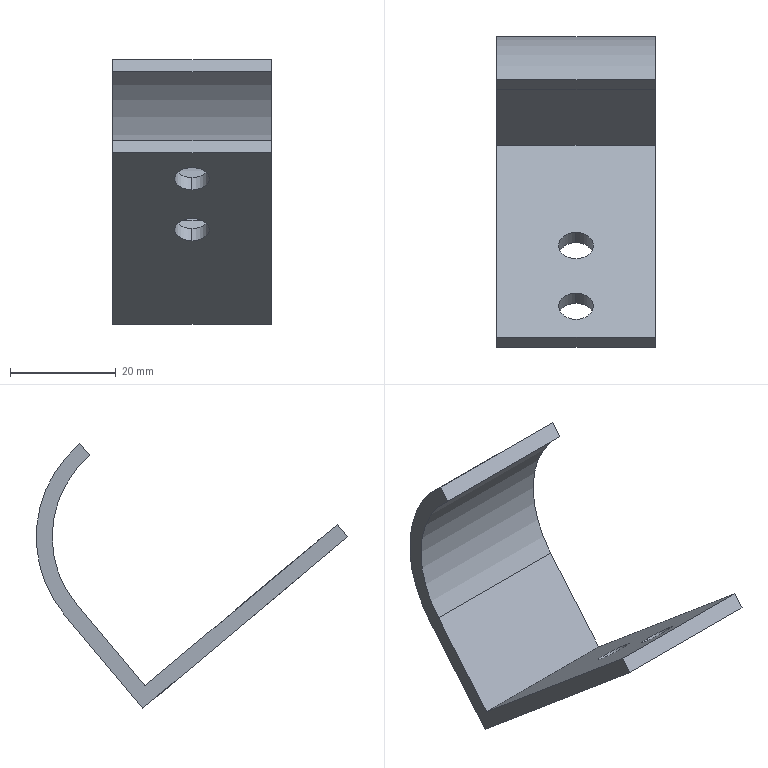Part | SolidWorks | features BaseBody 1 | 1 solid | 14 faces | box 30 x 58.835 x 50.022 mm | volume 9184 mm3 | plane 8 | cylinder 6 | commonest cylinder face diameters 6.5 x4 40 x1 46 x1
STEP:
#1=CARTESIAN_POINT('',(85.,219.284,-334.482));
#2=VERTEX_POINT('',#1);
#3=CARTESIAN_POINT('',(85.,224.263,-338.66));
#4=VERTEX_POINT('',#3);
#5=CARTESIAN_POINT('',(85.,221.774,-336.571));
#6=DIRECTION('',(0.,-0.6428,-0.766));
#7=DIRECTION('',(0.,-0.766,0.6428));
#8=AXIS2_PLACEMENT_3D('',#5,#6,#7);
#9=CIRCLE('',#8,3.25);
#10=EDGE_CURVE('',#2,#4,#9,.T.);
#11=ORIENTED_EDGE('',*,*,#10,.T.);
#12=CARTESIAN_POINT('',(85.,226.192,-336.362));
#13=VERTEX_POINT('',#12);
#14=CARTESIAN_POINT('',(85.,219.764,-344.023));
#15=DIRECTION('',(0.,0.6428,0.766));
#16=VECTOR('',#15,1000.);
#17=LINE('',#14,#16);
#18=EDGE_CURVE('',#4,#13,#17,.T.);
#19=ORIENTED_EDGE('',*,*,#18,.T.);
#20=CARTESIAN_POINT('',(85.,221.212,-332.184));
#21=VERTEX_POINT('',#20);
#22=CARTESIAN_POINT('',(85.,223.702,-334.273));
#23=DIRECTION('',(0.,-0.6428,-0.766));
#24=DIRECTION('',(0.,-0.766,0.6428));
#25=AXIS2_PLACEMENT_3D('',#22,#23,#24);
#26=CIRCLE('',#25,3.25);
#27=EDGE_CURVE('',#21,#13,#26,.T.);
#28=ORIENTED_EDGE('',*,*,#27,.F.);
#29=CARTESIAN_POINT('',(85.,214.785,-339.844));
#30=DIRECTION('',(0.,0.6428,0.766));
#31=VECTOR('',#30,1000.);
#32=LINE('',#29,#31);
#33=EDGE_CURVE('',#2,#21,#32,.T.);
#34=ORIENTED_EDGE('',*,*,#33,.F.);
#35=EDGE_LOOP('',(#11,#19,#28,#34));
#36=FACE_OUTER_BOUND('',#35,.T.);
#37=CARTESIAN_POINT('',(85.,217.274,-341.934));
#38=DIRECTION('',(0.,0.6428,0.766));
#39=DIRECTION('',(0.,-0.766,0.6428));
#40=AXIS2_PLACEMENT_3D('',#37,#38,#39);
#41=CYLINDRICAL_SURFACE('',#40,3.25);
#42=ADVANCED_FACE('',(#36),#41,.F.);
#43=CARTESIAN_POINT('',(85.,207.803,-324.848));
#44=VERTEX_POINT('',#43);
#45=CARTESIAN_POINT('',(85.,212.782,-329.026));
#46=VERTEX_POINT('',#45);
#47=CARTESIAN_POINT('',(85.,210.292,-326.937));
#48=DIRECTION('',(0.,-0.6428,-0.766));
#49=DIRECTION('',(0.,-0.766,0.6428));
#50=AXIS2_PLACEMENT_3D('',#47,#48,#49);
#51=CIRCLE('',#50,3.25);
#52=EDGE_CURVE('',#44,#46,#51,.T.);
#53=ORIENTED_EDGE('',*,*,#52,.T.);
#54=CARTESIAN_POINT('',(85.,214.71,-326.728));
#55=VERTEX_POINT('',#54);
#56=CARTESIAN_POINT('',(85.,208.282,-334.388));
#57=DIRECTION('',(0.,0.6428,0.766));
#58=VECTOR('',#57,1000.);
#59=LINE('',#56,#58);
#60=EDGE_CURVE('',#46,#55,#59,.T.);
#61=ORIENTED_EDGE('',*,*,#60,.T.);
#62=CARTESIAN_POINT('',(85.,209.731,-322.55));
#63=VERTEX_POINT('',#62);
#64=CARTESIAN_POINT('',(85.,212.221,-324.639));
#65=DIRECTION('',(0.,-0.6428,-0.766));
#66=DIRECTION('',(0.,-0.766,0.6428));
#67=AXIS2_PLACEMENT_3D('',#64,#65,#66);
#68=CIRCLE('',#67,3.25);
#69=EDGE_CURVE('',#63,#55,#68,.T.);
#70=ORIENTED_EDGE('',*,*,#69,.F.);
#71=CARTESIAN_POINT('',(85.,203.303,-330.21));
#72=DIRECTION('',(0.,0.6428,0.766));
#73=VECTOR('',#72,1000.);
#74=LINE('',#71,#73);
#75=EDGE_CURVE('',#44,#63,#74,.T.);
#76=ORIENTED_EDGE('',*,*,#75,.F.);
#77=EDGE_LOOP('',(#53,#61,#70,#76));
#78=FACE_OUTER_BOUND('',#77,.T.);
#79=CARTESIAN_POINT('',(85.,205.793,-332.299));
#80=DIRECTION('',(0.,0.6428,0.766));
#81=DIRECTION('',(0.,-0.766,0.6428));
#82=AXIS2_PLACEMENT_3D('',#79,#80,#81);
#83=CYLINDRICAL_SURFACE('',#82,3.25);
#84=ADVANCED_FACE('',(#78),#83,.F.);
#85=CARTESIAN_POINT('',(70.,204.42,-322.01));
#86=VERTEX_POINT('',#85);
#87=CARTESIAN_POINT('',(100.,204.42,-322.01));
#88=VERTEX_POINT('',#87);
#89=CARTESIAN_POINT('',(70.,204.42,-322.01));
#90=DIRECTION('',(1.,0.,0.));
#91=VECTOR('',#90,1000.);
#92=LINE('',#89,#91);
#93=EDGE_CURVE('',#86,#88,#92,.T.);
#94=ORIENTED_EDGE('',*,*,#93,.F.);
#95=CARTESIAN_POINT('',(70.,243.09,-354.458));
#96=VERTEX_POINT('',#95);
#97=CARTESIAN_POINT('',(70.,243.09,-354.458));
#98=DIRECTION('',(0.,-0.766,0.6428));
#99=VECTOR('',#98,1000.);
#100=LINE('',#97,#99);
#101=EDGE_CURVE('',#96,#86,#100,.T.);
#102=ORIENTED_EDGE('',*,*,#101,.F.);
#103=CARTESIAN_POINT('',(100.,243.09,-354.458));
#104=VERTEX_POINT('',#103);
#105=CARTESIAN_POINT('',(70.,243.09,-354.458));
#106=DIRECTION('',(-1.,0.,0.));
#107=VECTOR('',#106,1000.);
#108=LINE('',#105,#107);
#109=EDGE_CURVE('',#104,#96,#108,.T.);
#110=ORIENTED_EDGE('',*,*,#109,.F.);
#111=CARTESIAN_POINT('',(100.,243.09,-354.458));
#112=DIRECTION('',(0.,0.766,-0.6428));
#113=VECTOR('',#112,1000.);
#114=LINE('',#111,#113);
#115=EDGE_CURVE('',#88,#104,#114,.T.);
#116=ORIENTED_EDGE('',*,*,#115,.F.);
#117=EDGE_LOOP('',(#94,#102,#110,#116));
#118=FACE_OUTER_BOUND('',#117,.T.);
#119=ORIENTED_EDGE('',*,*,#10,.F.);
#120=CARTESIAN_POINT('',(85.,221.774,-336.571));
#121=DIRECTION('',(0.,-0.6428,-0.766));
#122=DIRECTION('',(0.,-0.766,0.6428));
#123=AXIS2_PLACEMENT_3D('',#120,#121,#122);
#124=CIRCLE('',#123,3.25);
#125=EDGE_CURVE('',#4,#2,#124,.T.);
#126=ORIENTED_EDGE('',*,*,#125,.F.);
#127=EDGE_LOOP('',(#119,#126));
#128=FACE_BOUND('',#127,.T.);
#129=ORIENTED_EDGE('',*,*,#52,.F.);
#130=CARTESIAN_POINT('',(85.,210.292,-326.937));
#131=DIRECTION('',(0.,-0.6428,-0.766));
#132=DIRECTION('',(0.,-0.766,0.6428));
#133=AXIS2_PLACEMENT_3D('',#130,#131,#132);
#134=CIRCLE('',#133,3.25);
#135=EDGE_CURVE('',#46,#44,#134,.T.);
#136=ORIENTED_EDGE('',*,*,#135,.F.);
#137=EDGE_LOOP('',(#129,#136));
#138=FACE_BOUND('',#137,.T.);
#139=CARTESIAN_POINT('',(70.,243.09,-354.458));
#140=DIRECTION('',(0.,0.6428,0.766));
#141=DIRECTION('',(0.,-0.766,0.6428));
#142=AXIS2_PLACEMENT_3D('',#139,#140,#141);
#143=PLANE('',#142);
#144=ADVANCED_FACE('',(#118,#128,#138),#143,.F.);
#145=CARTESIAN_POINT('',(100.,255.039,-304.436));
#146=VERTEX_POINT('',#145);
#147=CARTESIAN_POINT('',(100.,253.111,-306.734));
#148=VERTEX_POINT('',#147);
#149=CARTESIAN_POINT('',(100.,255.039,-304.436));
#150=DIRECTION('',(0.,-0.6428,-0.766));
#151=VECTOR('',#150,1000.);
#152=LINE('',#149,#151);
#153=EDGE_CURVE('',#146,#148,#152,.T.);
#154=ORIENTED_EDGE('',*,*,#153,.T.);
#155=CARTESIAN_POINT('',(100.,255.576,-334.91));
#156=VERTEX_POINT('',#155);
#157=CARTESIAN_POINT('',(100.,240.255,-322.055));
#158=DIRECTION('',(-1.,0.,0.));
#159=DIRECTION('',(0.,0.,-1.));
#160=AXIS2_PLACEMENT_3D('',#157,#158,#159);
#161=CIRCLE('',#160,20.);
#162=EDGE_CURVE('',#148,#156,#161,.T.);
#163=ORIENTED_EDGE('',*,*,#162,.T.);
#164=CARTESIAN_POINT('',(100.,242.72,-350.231));
#165=VERTEX_POINT('',#164);
#166=CARTESIAN_POINT('',(100.,255.576,-334.91));
#167=DIRECTION('',(0.,-0.6428,-0.766));
#168=VECTOR('',#167,1000.);
#169=LINE('',#166,#168);
#170=EDGE_CURVE('',#156,#165,#169,.T.);
#171=ORIENTED_EDGE('',*,*,#170,.T.);
#172=CARTESIAN_POINT('',(100.,206.349,-319.712));
#173=VERTEX_POINT('',#172);
#174=CARTESIAN_POINT('',(100.,242.72,-350.231));
#175=DIRECTION('',(0.,-0.766,0.6428));
#176=VECTOR('',#175,1000.);
#177=LINE('',#174,#176);
#178=EDGE_CURVE('',#165,#173,#177,.T.);
#179=ORIENTED_EDGE('',*,*,#178,.T.);
#180=CARTESIAN_POINT('',(100.,206.349,-319.712));
#181=DIRECTION('',(0.,-0.6428,-0.766));
#182=VECTOR('',#181,1000.);
#183=LINE('',#180,#182);
#184=EDGE_CURVE('',#173,#88,#183,.T.);
#185=ORIENTED_EDGE('',*,*,#184,.T.);
#186=ORIENTED_EDGE('',*,*,#115,.T.);
#187=CARTESIAN_POINT('',(100.,257.874,-336.839));
#188=VERTEX_POINT('',#187);
#189=CARTESIAN_POINT('',(100.,243.09,-354.458));
#190=DIRECTION('',(0.,0.6428,0.766));
#191=VECTOR('',#190,1000.);
#192=LINE('',#189,#191);
#193=EDGE_CURVE('',#104,#188,#192,.T.);
#194=ORIENTED_EDGE('',*,*,#193,.T.);
#195=CARTESIAN_POINT('',(100.,240.255,-322.055));
#196=DIRECTION('',(1.,0.,0.));
#197=DIRECTION('',(0.,0.,-1.));
#198=AXIS2_PLACEMENT_3D('',#195,#196,#197);
#199=CIRCLE('',#198,23.);
#200=EDGE_CURVE('',#188,#146,#199,.T.);
#201=ORIENTED_EDGE('',*,*,#200,.T.);
#202=EDGE_LOOP('',(#154,#163,#171,#179,#185,#186,#194,#201));
#203=FACE_OUTER_BOUND('',#202,.T.);
#204=CARTESIAN_POINT('',(100.,240.255,-322.055));
#205=DIRECTION('',(1.,0.,0.));
#206=DIRECTION('',(0.,0.,-1.));
#207=AXIS2_PLACEMENT_3D('',#204,#205,#206);
#208=PLANE('',#207);
#209=ADVANCED_FACE('',(#203),#208,.T.);
#210=CARTESIAN_POINT('',(70.,206.349,-319.712));
#211=VERTEX_POINT('',#210);
#212=CARTESIAN_POINT('',(70.,206.349,-319.712));
#213=DIRECTION('',(1.,0.,0.));
#214=VECTOR('',#213,1000.);
#215=LINE('',#212,#214);
#216=EDGE_CURVE('',#211,#173,#215,.T.);
#217=ORIENTED_EDGE('',*,*,#216,.F.);
#218=CARTESIAN_POINT('',(70.,206.349,-319.712));
#219=DIRECTION('',(0.,0.6428,0.766));
#220=VECTOR('',#219,1000.);
#221=LINE('',#218,#220);
#222=EDGE_CURVE('',#86,#211,#221,.T.);
#223=ORIENTED_EDGE('',*,*,#222,.F.);
#224=ORIENTED_EDGE('',*,*,#93,.T.);
#225=ORIENTED_EDGE('',*,*,#184,.F.);
#226=EDGE_LOOP('',(#217,#223,#224,#225));
#227=FACE_OUTER_BOUND('',#226,.T.);
#228=CARTESIAN_POINT('',(70.,206.349,-319.712));
#229=DIRECTION('',(0.,0.766,-0.6428));
#230=DIRECTION('',(0.,0.6428,0.766));
#231=AXIS2_PLACEMENT_3D('',#228,#229,#230);
#232=PLANE('',#231);
#233=ADVANCED_FACE('',(#227),#232,.F.);
#234=CARTESIAN_POINT('',(70.,253.111,-306.734));
#235=VERTEX_POINT('',#234);
#236=CARTESIAN_POINT('',(70.,255.576,-334.91));
#237=VERTEX_POINT('',#236);
#238=CARTESIAN_POINT('',(70.,240.255,-322.055));
#239=DIRECTION('',(-1.,0.,0.));
#240=DIRECTION('',(0.,0.,-1.));
#241=AXIS2_PLACEMENT_3D('',#238,#239,#240);
#242=CIRCLE('',#241,20.);
#243=EDGE_CURVE('',#235,#237,#242,.T.);
#244=ORIENTED_EDGE('',*,*,#243,.F.);
#245=CARTESIAN_POINT('',(70.,255.039,-304.436));
#246=VERTEX_POINT('',#245);
#247=CARTESIAN_POINT('',(70.,255.039,-304.436));
#248=DIRECTION('',(0.,-0.6428,-0.766));
#249=VECTOR('',#248,1000.);
#250=LINE('',#247,#249);
#251=EDGE_CURVE('',#246,#235,#250,.T.);
#252=ORIENTED_EDGE('',*,*,#251,.F.);
#253=CARTESIAN_POINT('',(70.,257.874,-336.839));
#254=VERTEX_POINT('',#253);
#255=CARTESIAN_POINT('',(70.,240.255,-322.055));
#256=DIRECTION('',(1.,0.,0.));
#257=DIRECTION('',(0.,0.,-1.));
#258=AXIS2_PLACEMENT_3D('',#255,#256,#257);
#259=CIRCLE('',#258,23.);
#260=EDGE_CURVE('',#254,#246,#259,.T.);
#261=ORIENTED_EDGE('',*,*,#260,.F.);
#262=CARTESIAN_POINT('',(70.,243.09,-354.458));
#263=DIRECTION('',(0.,0.6428,0.766));
#264=VECTOR('',#263,1000.);
#265=LINE('',#262,#264);
#266=EDGE_CURVE('',#96,#254,#265,.T.);
#267=ORIENTED_EDGE('',*,*,#266,.F.);
#268=ORIENTED_EDGE('',*,*,#101,.T.);
#269=ORIENTED_EDGE('',*,*,#222,.T.);
#270=CARTESIAN_POINT('',(70.,242.72,-350.231));
#271=VERTEX_POINT('',#270);
#272=CARTESIAN_POINT('',(70.,242.72,-350.231));
#273=DIRECTION('',(0.,-0.766,0.6428));
#274=VECTOR('',#273,1000.);
#275=LINE('',#272,#274);
#276=EDGE_CURVE('',#271,#211,#275,.T.);
#277=ORIENTED_EDGE('',*,*,#276,.F.);
#278=CARTESIAN_POINT('',(70.,255.576,-334.91));
#279=DIRECTION('',(0.,-0.6428,-0.766));
#280=VECTOR('',#279,1000.);
#281=LINE('',#278,#280);
#282=EDGE_CURVE('',#237,#271,#281,.T.);
#283=ORIENTED_EDGE('',*,*,#282,.F.);
#284=EDGE_LOOP('',(#244,#252,#261,#267,#268,#269,#277,#283));
#285=FACE_OUTER_BOUND('',#284,.T.);
#286=CARTESIAN_POINT('',(70.,240.255,-322.055));
#287=DIRECTION('',(1.,0.,0.));
#288=DIRECTION('',(0.,0.,-1.));
#289=AXIS2_PLACEMENT_3D('',#286,#287,#288);
#290=PLANE('',#289);
#291=ADVANCED_FACE('',(#285),#290,.F.);
#292=ORIENTED_EDGE('',*,*,#109,.T.);
#293=ORIENTED_EDGE('',*,*,#266,.T.);
#294=CARTESIAN_POINT('',(70.,257.874,-336.839));
#295=DIRECTION('',(-1.,0.,0.));
#296=VECTOR('',#295,1000.);
#297=LINE('',#294,#296);
#298=EDGE_CURVE('',#188,#254,#297,.T.);
#299=ORIENTED_EDGE('',*,*,#298,.F.);
#300=ORIENTED_EDGE('',*,*,#193,.F.);
#301=EDGE_LOOP('',(#292,#293,#299,#300));
#302=FACE_OUTER_BOUND('',#301,.T.);
#303=CARTESIAN_POINT('',(70.,243.09,-354.458));
#304=DIRECTION('',(0.,-0.766,0.6428));
#305=DIRECTION('',(0.,-0.6428,-0.766));
#306=AXIS2_PLACEMENT_3D('',#303,#304,#305);
#307=PLANE('',#306);
#308=ADVANCED_FACE('',(#302),#307,.F.);
#309=ORIENTED_EDGE('',*,*,#18,.F.);
#310=ORIENTED_EDGE('',*,*,#125,.T.);
#311=ORIENTED_EDGE('',*,*,#33,.T.);
#312=CARTESIAN_POINT('',(85.,223.702,-334.273));
#313=DIRECTION('',(0.,-0.6428,-0.766));
#314=DIRECTION('',(0.,-0.766,0.6428));
#315=AXIS2_PLACEMENT_3D('',#312,#313,#314);
#316=CIRCLE('',#315,3.25);
#317=EDGE_CURVE('',#13,#21,#316,.T.);
#318=ORIENTED_EDGE('',*,*,#317,.F.);
#319=EDGE_LOOP('',(#309,#310,#311,#318));
#320=FACE_OUTER_BOUND('',#319,.T.);
#321=CARTESIAN_POINT('',(85.,217.274,-341.934));
#322=DIRECTION('',(0.,0.6428,0.766));
#323=DIRECTION('',(0.,-0.766,0.6428));
#324=AXIS2_PLACEMENT_3D('',#321,#322,#323);
#325=CYLINDRICAL_SURFACE('',#324,3.25);
#326=ADVANCED_FACE('',(#320),#325,.F.);
#327=ORIENTED_EDGE('',*,*,#60,.F.);
#328=ORIENTED_EDGE('',*,*,#135,.T.);
#329=ORIENTED_EDGE('',*,*,#75,.T.);
#330=CARTESIAN_POINT('',(85.,212.221,-324.639));
#331=DIRECTION('',(0.,-0.6428,-0.766));
#332=DIRECTION('',(0.,-0.766,0.6428));
#333=AXIS2_PLACEMENT_3D('',#330,#331,#332);
#334=CIRCLE('',#333,3.25);
#335=EDGE_CURVE('',#55,#63,#334,.T.);
#336=ORIENTED_EDGE('',*,*,#335,.F.);
#337=EDGE_LOOP('',(#327,#328,#329,#336));
#338=FACE_OUTER_BOUND('',#337,.T.);
#339=CARTESIAN_POINT('',(85.,205.793,-332.299));
#340=DIRECTION('',(0.,0.6428,0.766));
#341=DIRECTION('',(0.,-0.766,0.6428));
#342=AXIS2_PLACEMENT_3D('',#339,#340,#341);
#343=CYLINDRICAL_SURFACE('',#342,3.25);
#344=ADVANCED_FACE('',(#338),#343,.F.);
#345=CARTESIAN_POINT('',(70.,253.111,-306.734));
#346=DIRECTION('',(1.,0.,0.));
#347=VECTOR('',#346,1000.);
#348=LINE('',#345,#347);
#349=EDGE_CURVE('',#235,#148,#348,.T.);
#350=ORIENTED_EDGE('',*,*,#349,.F.);
#351=ORIENTED_EDGE('',*,*,#243,.T.);
#352=CARTESIAN_POINT('',(70.,255.576,-334.91));
#353=DIRECTION('',(-1.,0.,0.));
#354=VECTOR('',#353,1000.);
#355=LINE('',#352,#354);
#356=EDGE_CURVE('',#156,#237,#355,.T.);
#357=ORIENTED_EDGE('',*,*,#356,.F.);
#358=ORIENTED_EDGE('',*,*,#162,.F.);
#359=EDGE_LOOP('',(#350,#351,#357,#358));
#360=FACE_OUTER_BOUND('',#359,.T.);
#361=CARTESIAN_POINT('',(70.,240.255,-322.055));
#362=DIRECTION('',(1.,0.,0.));
#363=DIRECTION('',(0.,0.,-1.));
#364=AXIS2_PLACEMENT_3D('',#361,#362,#363);
#365=CYLINDRICAL_SURFACE('',#364,20.);
#366=ADVANCED_FACE('',(#360),#365,.F.);
#367=CARTESIAN_POINT('',(70.,255.039,-304.436));
#368=DIRECTION('',(1.,0.,0.));
#369=VECTOR('',#368,1000.);
#370=LINE('',#367,#369);
#371=EDGE_CURVE('',#246,#146,#370,.T.);
#372=ORIENTED_EDGE('',*,*,#371,.F.);
#373=ORIENTED_EDGE('',*,*,#251,.T.);
#374=ORIENTED_EDGE('',*,*,#349,.T.);
#375=ORIENTED_EDGE('',*,*,#153,.F.);
#376=EDGE_LOOP('',(#372,#373,#374,#375));
#377=FACE_OUTER_BOUND('',#376,.T.);
#378=CARTESIAN_POINT('',(70.,253.111,-306.734));
#379=DIRECTION('',(0.,0.766,-0.6428));
#380=DIRECTION('',(0.,0.6428,0.766));
#381=AXIS2_PLACEMENT_3D('',#378,#379,#380);
#382=PLANE('',#381);
#383=ADVANCED_FACE('',(#377),#382,.F.);
#384=ORIENTED_EDGE('',*,*,#260,.T.);
#385=ORIENTED_EDGE('',*,*,#371,.T.);
#386=ORIENTED_EDGE('',*,*,#200,.F.);
#387=ORIENTED_EDGE('',*,*,#298,.T.);
#388=EDGE_LOOP('',(#384,#385,#386,#387));
#389=FACE_OUTER_BOUND('',#388,.T.);
#390=CARTESIAN_POINT('',(70.,240.255,-322.055));
#391=DIRECTION('',(1.,0.,0.));
#392=DIRECTION('',(0.,0.,-1.));
#393=AXIS2_PLACEMENT_3D('',#390,#391,#392);
#394=CYLINDRICAL_SURFACE('',#393,23.);
#395=ADVANCED_FACE('',(#389),#394,.T.);
#396=CARTESIAN_POINT('',(70.,242.72,-350.231));
#397=DIRECTION('',(1.,0.,0.));
#398=VECTOR('',#397,1000.);
#399=LINE('',#396,#398);
#400=EDGE_CURVE('',#271,#165,#399,.T.);
#401=ORIENTED_EDGE('',*,*,#400,.F.);
#402=ORIENTED_EDGE('',*,*,#276,.T.);
#403=ORIENTED_EDGE('',*,*,#216,.T.);
#404=ORIENTED_EDGE('',*,*,#178,.F.);
#405=EDGE_LOOP('',(#401,#402,#403,#404));
#406=FACE_OUTER_BOUND('',#405,.T.);
#407=ORIENTED_EDGE('',*,*,#27,.T.);
#408=ORIENTED_EDGE('',*,*,#317,.T.);
#409=EDGE_LOOP('',(#407,#408));
#410=FACE_BOUND('',#409,.T.);
#411=ORIENTED_EDGE('',*,*,#69,.T.);
#412=ORIENTED_EDGE('',*,*,#335,.T.);
#413=EDGE_LOOP('',(#411,#412));
#414=FACE_BOUND('',#413,.T.);
#415=CARTESIAN_POINT('',(70.,242.72,-350.231));
#416=DIRECTION('',(0.,-0.6428,-0.766));
#417=DIRECTION('',(0.,0.766,-0.6428));
#418=AXIS2_PLACEMENT_3D('',#415,#416,#417);
#419=PLANE('',#418);
#420=ADVANCED_FACE('',(#406,#410,#414),#419,.F.);
#421=ORIENTED_EDGE('',*,*,#356,.T.);
#422=ORIENTED_EDGE('',*,*,#282,.T.);
#423=ORIENTED_EDGE('',*,*,#400,.T.);
#424=ORIENTED_EDGE('',*,*,#170,.F.);
#425=EDGE_LOOP('',(#421,#422,#423,#424));
#426=FACE_OUTER_BOUND('',#425,.T.);
#427=CARTESIAN_POINT('',(70.,242.72,-350.231));
#428=DIRECTION('',(0.,0.766,-0.6428));
#429=DIRECTION('',(0.,0.6428,0.766));
#430=AXIS2_PLACEMENT_3D('',#427,#428,#429);
#431=PLANE('',#430);
#432=ADVANCED_FACE('',(#426),#431,.F.);
#433=CLOSED_SHELL('',(#42,#84,#144,#209,#233,#291,#308,#326,#344,#366,#383,#395,#420,#432));
#434=MANIFOLD_SOLID_BREP('',#433);
#435=CARTESIAN_POINT('',(0.,0.,0.));
#436=DIRECTION('',(0.,0.,1.));
#437=DIRECTION('',(1.,0.,0.));
#438=AXIS2_PLACEMENT_3D('',#435,#436,#437);
#439=(LENGTH_UNIT()NAMED_UNIT(*)SI_UNIT(.MILLI.,.METRE.));
#440=UNCERTAINTY_MEASURE_WITH_UNIT(LENGTH_MEASURE(0.00001),#439,'','');
#441=(NAMED_UNIT(*)PLANE_ANGLE_UNIT()SI_UNIT($,.RADIAN.));
#442=(NAMED_UNIT(*)SI_UNIT($,.STERADIAN.)SOLID_ANGLE_UNIT());
#443=(GEOMETRIC_REPRESENTATION_CONTEXT(3)GLOBAL_UNCERTAINTY_ASSIGNED_CONTEXT((#440))GLOBAL_UNIT_ASSIGNED_CONTEXT((#439,#441,#442))REPRESENTATION_CONTEXT('',''));
#444=ADVANCED_BREP_SHAPE_REPRESENTATION('',(#434,#438),#443);